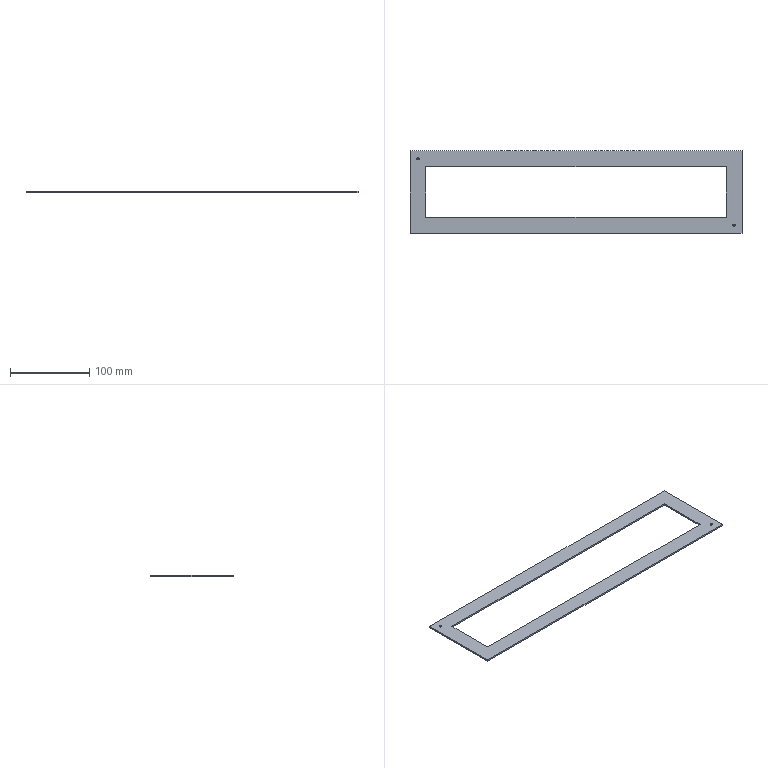Part | STEP file | Trunking Spacer Plate | 1 solid | 14 faces | box 420 x 104 x 2 mm | volume 38692 mm3 | plane 10 | cylinder 4 | commonest cylinder face diameters 3 x4
STEP:
#1=CARTESIAN_POINT('',(1421.716,-975.567,-2.));
#2=VERTEX_POINT('',#1);
#3=CARTESIAN_POINT('',(1418.716,-975.567,-2.));
#4=VERTEX_POINT('',#3);
#5=CARTESIAN_POINT('',(1420.216,-975.567,-2.));
#6=DIRECTION('',(0.,0.,-1.));
#7=DIRECTION('',(1.,0.,0.));
#8=AXIS2_PLACEMENT_3D('',#5,#6,#7);
#9=CIRCLE('',#8,1.5);
#10=EDGE_CURVE('',#2,#4,#9,.T.);
#11=ORIENTED_EDGE('',*,*,#10,.T.);
#12=CARTESIAN_POINT('',(1418.716,-975.567,0.));
#13=VERTEX_POINT('',#12);
#14=CARTESIAN_POINT('',(1418.716,-975.567,-2.));
#15=DIRECTION('',(0.,0.,1.));
#16=VECTOR('',#15,1000.);
#17=LINE('',#14,#16);
#18=EDGE_CURVE('',#4,#13,#17,.T.);
#19=ORIENTED_EDGE('',*,*,#18,.T.);
#20=CARTESIAN_POINT('',(1421.716,-975.567,0.));
#21=VERTEX_POINT('',#20);
#22=CARTESIAN_POINT('',(1420.216,-975.567,0.));
#23=DIRECTION('',(0.,0.,-1.));
#24=DIRECTION('',(1.,0.,0.));
#25=AXIS2_PLACEMENT_3D('',#22,#23,#24);
#26=CIRCLE('',#25,1.5);
#27=EDGE_CURVE('',#21,#13,#26,.T.);
#28=ORIENTED_EDGE('',*,*,#27,.F.);
#29=CARTESIAN_POINT('',(1421.716,-975.567,-2.));
#30=DIRECTION('',(0.,0.,1.));
#31=VECTOR('',#30,1000.);
#32=LINE('',#29,#31);
#33=EDGE_CURVE('',#2,#21,#32,.T.);
#34=ORIENTED_EDGE('',*,*,#33,.F.);
#35=EDGE_LOOP('',(#11,#19,#28,#34));
#36=FACE_OUTER_BOUND('',#35,.T.);
#37=CARTESIAN_POINT('',(1420.216,-975.567,-2.));
#38=DIRECTION('',(0.,0.,1.));
#39=DIRECTION('',(1.,0.,0.));
#40=AXIS2_PLACEMENT_3D('',#37,#38,#39);
#41=CYLINDRICAL_SURFACE('',#40,1.5);
#42=ADVANCED_FACE('',(#36),#41,.F.);
#43=CARTESIAN_POINT('',(1021.716,-891.567,-2.));
#44=VERTEX_POINT('',#43);
#45=CARTESIAN_POINT('',(1018.716,-891.567,-2.));
#46=VERTEX_POINT('',#45);
#47=CARTESIAN_POINT('',(1020.216,-891.567,-2.));
#48=DIRECTION('',(0.,0.,-1.));
#49=DIRECTION('',(1.,0.,0.));
#50=AXIS2_PLACEMENT_3D('',#47,#48,#49);
#51=CIRCLE('',#50,1.5);
#52=EDGE_CURVE('',#44,#46,#51,.T.);
#53=ORIENTED_EDGE('',*,*,#52,.T.);
#54=CARTESIAN_POINT('',(1018.716,-891.567,0.));
#55=VERTEX_POINT('',#54);
#56=CARTESIAN_POINT('',(1018.716,-891.567,-2.));
#57=DIRECTION('',(0.,0.,1.));
#58=VECTOR('',#57,1000.);
#59=LINE('',#56,#58);
#60=EDGE_CURVE('',#46,#55,#59,.T.);
#61=ORIENTED_EDGE('',*,*,#60,.T.);
#62=CARTESIAN_POINT('',(1021.716,-891.567,0.));
#63=VERTEX_POINT('',#62);
#64=CARTESIAN_POINT('',(1020.216,-891.567,0.));
#65=DIRECTION('',(0.,0.,-1.));
#66=DIRECTION('',(1.,0.,0.));
#67=AXIS2_PLACEMENT_3D('',#64,#65,#66);
#68=CIRCLE('',#67,1.5);
#69=EDGE_CURVE('',#63,#55,#68,.T.);
#70=ORIENTED_EDGE('',*,*,#69,.F.);
#71=CARTESIAN_POINT('',(1021.716,-891.567,-2.));
#72=DIRECTION('',(0.,0.,1.));
#73=VECTOR('',#72,1000.);
#74=LINE('',#71,#73);
#75=EDGE_CURVE('',#44,#63,#74,.T.);
#76=ORIENTED_EDGE('',*,*,#75,.F.);
#77=EDGE_LOOP('',(#53,#61,#70,#76));
#78=FACE_OUTER_BOUND('',#77,.T.);
#79=CARTESIAN_POINT('',(1020.216,-891.567,-2.));
#80=DIRECTION('',(0.,0.,1.));
#81=DIRECTION('',(1.,0.,0.));
#82=AXIS2_PLACEMENT_3D('',#79,#80,#81);
#83=CYLINDRICAL_SURFACE('',#82,1.5);
#84=ADVANCED_FACE('',(#78),#83,.F.);
#85=CARTESIAN_POINT('',(1430.216,-881.567,-2.));
#86=VERTEX_POINT('',#85);
#87=CARTESIAN_POINT('',(1010.216,-881.567,-2.));
#88=VERTEX_POINT('',#87);
#89=CARTESIAN_POINT('',(0.,-881.567,-2.));
#90=DIRECTION('',(-1.,0.,0.));
#91=VECTOR('',#90,1000.);
#92=LINE('',#89,#91);
#93=EDGE_CURVE('',#86,#88,#92,.T.);
#94=ORIENTED_EDGE('',*,*,#93,.F.);
#95=CARTESIAN_POINT('',(1430.216,-985.567,-2.));
#96=VERTEX_POINT('',#95);
#97=CARTESIAN_POINT('',(1430.216,0.,-2.));
#98=DIRECTION('',(0.,1.,0.));
#99=VECTOR('',#98,1000.);
#100=LINE('',#97,#99);
#101=EDGE_CURVE('',#96,#86,#100,.T.);
#102=ORIENTED_EDGE('',*,*,#101,.F.);
#103=CARTESIAN_POINT('',(1010.216,-985.567,-2.));
#104=VERTEX_POINT('',#103);
#105=CARTESIAN_POINT('',(0.,-985.567,-2.));
#106=DIRECTION('',(1.,0.,0.));
#107=VECTOR('',#106,1000.);
#108=LINE('',#105,#107);
#109=EDGE_CURVE('',#104,#96,#108,.T.);
#110=ORIENTED_EDGE('',*,*,#109,.F.);
#111=CARTESIAN_POINT('',(1010.216,0.,-2.));
#112=DIRECTION('',(0.,-1.,0.));
#113=VECTOR('',#112,1000.);
#114=LINE('',#111,#113);
#115=EDGE_CURVE('',#88,#104,#114,.T.);
#116=ORIENTED_EDGE('',*,*,#115,.F.);
#117=EDGE_LOOP('',(#94,#102,#110,#116));
#118=FACE_OUTER_BOUND('',#117,.T.);
#119=ORIENTED_EDGE('',*,*,#10,.F.);
#120=CARTESIAN_POINT('',(1420.216,-975.567,-2.));
#121=DIRECTION('',(0.,0.,-1.));
#122=DIRECTION('',(1.,0.,0.));
#123=AXIS2_PLACEMENT_3D('',#120,#121,#122);
#124=CIRCLE('',#123,1.5);
#125=EDGE_CURVE('',#4,#2,#124,.T.);
#126=ORIENTED_EDGE('',*,*,#125,.F.);
#127=EDGE_LOOP('',(#119,#126));
#128=FACE_BOUND('',#127,.T.);
#129=ORIENTED_EDGE('',*,*,#52,.F.);
#130=CARTESIAN_POINT('',(1020.216,-891.567,-2.));
#131=DIRECTION('',(0.,0.,-1.));
#132=DIRECTION('',(1.,0.,0.));
#133=AXIS2_PLACEMENT_3D('',#130,#131,#132);
#134=CIRCLE('',#133,1.5);
#135=EDGE_CURVE('',#46,#44,#134,.T.);
#136=ORIENTED_EDGE('',*,*,#135,.F.);
#137=EDGE_LOOP('',(#129,#136));
#138=FACE_BOUND('',#137,.T.);
#139=CARTESIAN_POINT('',(1030.216,-965.567,-2.));
#140=VERTEX_POINT('',#139);
#141=CARTESIAN_POINT('',(1030.216,-901.567,-2.));
#142=VERTEX_POINT('',#141);
#143=CARTESIAN_POINT('',(1030.216,0.,-2.));
#144=DIRECTION('',(0.,1.,0.));
#145=VECTOR('',#144,1000.);
#146=LINE('',#143,#145);
#147=EDGE_CURVE('',#140,#142,#146,.T.);
#148=ORIENTED_EDGE('',*,*,#147,.F.);
#149=CARTESIAN_POINT('',(1410.216,-965.567,-2.));
#150=VERTEX_POINT('',#149);
#151=CARTESIAN_POINT('',(0.,-965.567,-2.));
#152=DIRECTION('',(-1.,0.,0.));
#153=VECTOR('',#152,1000.);
#154=LINE('',#151,#153);
#155=EDGE_CURVE('',#150,#140,#154,.T.);
#156=ORIENTED_EDGE('',*,*,#155,.F.);
#157=CARTESIAN_POINT('',(1410.216,-901.567,-2.));
#158=VERTEX_POINT('',#157);
#159=CARTESIAN_POINT('',(1410.216,0.,-2.));
#160=DIRECTION('',(0.,-1.,0.));
#161=VECTOR('',#160,1000.);
#162=LINE('',#159,#161);
#163=EDGE_CURVE('',#158,#150,#162,.T.);
#164=ORIENTED_EDGE('',*,*,#163,.F.);
#165=CARTESIAN_POINT('',(0.,-901.567,-2.));
#166=DIRECTION('',(1.,0.,0.));
#167=VECTOR('',#166,1000.);
#168=LINE('',#165,#167);
#169=EDGE_CURVE('',#142,#158,#168,.T.);
#170=ORIENTED_EDGE('',*,*,#169,.F.);
#171=EDGE_LOOP('',(#148,#156,#164,#170));
#172=FACE_BOUND('',#171,.T.);
#173=CARTESIAN_POINT('',(0.,0.,-2.));
#174=DIRECTION('',(0.,0.,1.));
#175=DIRECTION('',(1.,0.,0.));
#176=AXIS2_PLACEMENT_3D('',#173,#174,#175);
#177=PLANE('',#176);
#178=ADVANCED_FACE('',(#118,#128,#138,#172),#177,.F.);
#179=ORIENTED_EDGE('',*,*,#115,.T.);
#180=CARTESIAN_POINT('',(1010.216,-985.567,0.));
#181=VERTEX_POINT('',#180);
#182=CARTESIAN_POINT('',(1010.216,-985.567,-2.));
#183=DIRECTION('',(0.,0.,1.));
#184=VECTOR('',#183,1000.);
#185=LINE('',#182,#184);
#186=EDGE_CURVE('',#104,#181,#185,.T.);
#187=ORIENTED_EDGE('',*,*,#186,.T.);
#188=CARTESIAN_POINT('',(1010.216,-881.567,0.));
#189=VERTEX_POINT('',#188);
#190=CARTESIAN_POINT('',(1010.216,-881.567,0.));
#191=DIRECTION('',(0.,1.,0.));
#192=VECTOR('',#191,1000.);
#193=LINE('',#190,#192);
#194=EDGE_CURVE('',#181,#189,#193,.T.);
#195=ORIENTED_EDGE('',*,*,#194,.T.);
#196=CARTESIAN_POINT('',(1010.216,-881.567,-2.));
#197=DIRECTION('',(0.,0.,-1.));
#198=VECTOR('',#197,1000.);
#199=LINE('',#196,#198);
#200=EDGE_CURVE('',#189,#88,#199,.T.);
#201=ORIENTED_EDGE('',*,*,#200,.T.);
#202=EDGE_LOOP('',(#179,#187,#195,#201));
#203=FACE_OUTER_BOUND('',#202,.T.);
#204=CARTESIAN_POINT('',(1010.216,-881.567,-2.));
#205=DIRECTION('',(-1.,0.,0.));
#206=DIRECTION('',(0.,-1.,0.));
#207=AXIS2_PLACEMENT_3D('',#204,#205,#206);
#208=PLANE('',#207);
#209=ADVANCED_FACE('',(#203),#208,.T.);
#210=ORIENTED_EDGE('',*,*,#93,.T.);
#211=ORIENTED_EDGE('',*,*,#200,.F.);
#212=CARTESIAN_POINT('',(1430.216,-881.567,0.));
#213=VERTEX_POINT('',#212);
#214=CARTESIAN_POINT('',(1010.216,-881.567,0.));
#215=DIRECTION('',(1.,0.,0.));
#216=VECTOR('',#215,1000.);
#217=LINE('',#214,#216);
#218=EDGE_CURVE('',#189,#213,#217,.T.);
#219=ORIENTED_EDGE('',*,*,#218,.T.);
#220=CARTESIAN_POINT('',(1430.216,-881.567,-2.));
#221=DIRECTION('',(0.,0.,-1.));
#222=VECTOR('',#221,1000.);
#223=LINE('',#220,#222);
#224=EDGE_CURVE('',#213,#86,#223,.T.);
#225=ORIENTED_EDGE('',*,*,#224,.T.);
#226=EDGE_LOOP('',(#210,#211,#219,#225));
#227=FACE_OUTER_BOUND('',#226,.T.);
#228=CARTESIAN_POINT('',(1010.216,-881.567,-2.));
#229=DIRECTION('',(0.,1.,0.));
#230=DIRECTION('',(0.,0.,1.));
#231=AXIS2_PLACEMENT_3D('',#228,#229,#230);
#232=PLANE('',#231);
#233=ADVANCED_FACE('',(#227),#232,.T.);
#234=ORIENTED_EDGE('',*,*,#101,.T.);
#235=ORIENTED_EDGE('',*,*,#224,.F.);
#236=CARTESIAN_POINT('',(1430.216,-985.567,0.));
#237=VERTEX_POINT('',#236);
#238=CARTESIAN_POINT('',(1430.216,-881.567,0.));
#239=DIRECTION('',(0.,-1.,0.));
#240=VECTOR('',#239,1000.);
#241=LINE('',#238,#240);
#242=EDGE_CURVE('',#213,#237,#241,.T.);
#243=ORIENTED_EDGE('',*,*,#242,.T.);
#244=CARTESIAN_POINT('',(1430.216,-985.567,-2.));
#245=DIRECTION('',(0.,0.,-1.));
#246=VECTOR('',#245,1000.);
#247=LINE('',#244,#246);
#248=EDGE_CURVE('',#237,#96,#247,.T.);
#249=ORIENTED_EDGE('',*,*,#248,.T.);
#250=EDGE_LOOP('',(#234,#235,#243,#249));
#251=FACE_OUTER_BOUND('',#250,.T.);
#252=CARTESIAN_POINT('',(1430.216,-881.567,-2.));
#253=DIRECTION('',(1.,0.,0.));
#254=DIRECTION('',(0.,1.,0.));
#255=AXIS2_PLACEMENT_3D('',#252,#253,#254);
#256=PLANE('',#255);
#257=ADVANCED_FACE('',(#251),#256,.T.);
#258=ORIENTED_EDGE('',*,*,#109,.T.);
#259=ORIENTED_EDGE('',*,*,#248,.F.);
#260=CARTESIAN_POINT('',(1010.216,-985.567,0.));
#261=DIRECTION('',(-1.,0.,0.));
#262=VECTOR('',#261,1000.);
#263=LINE('',#260,#262);
#264=EDGE_CURVE('',#237,#181,#263,.T.);
#265=ORIENTED_EDGE('',*,*,#264,.T.);
#266=ORIENTED_EDGE('',*,*,#186,.F.);
#267=EDGE_LOOP('',(#258,#259,#265,#266));
#268=FACE_OUTER_BOUND('',#267,.T.);
#269=CARTESIAN_POINT('',(1010.216,-985.567,-2.));
#270=DIRECTION('',(0.,-1.,0.));
#271=DIRECTION('',(0.,0.,-1.));
#272=AXIS2_PLACEMENT_3D('',#269,#270,#271);
#273=PLANE('',#272);
#274=ADVANCED_FACE('',(#268),#273,.T.);
#275=ORIENTED_EDGE('',*,*,#18,.F.);
#276=ORIENTED_EDGE('',*,*,#125,.T.);
#277=ORIENTED_EDGE('',*,*,#33,.T.);
#278=CARTESIAN_POINT('',(1420.216,-975.567,0.));
#279=DIRECTION('',(0.,0.,-1.));
#280=DIRECTION('',(1.,0.,0.));
#281=AXIS2_PLACEMENT_3D('',#278,#279,#280);
#282=CIRCLE('',#281,1.5);
#283=EDGE_CURVE('',#13,#21,#282,.T.);
#284=ORIENTED_EDGE('',*,*,#283,.F.);
#285=EDGE_LOOP('',(#275,#276,#277,#284));
#286=FACE_OUTER_BOUND('',#285,.T.);
#287=CARTESIAN_POINT('',(1420.216,-975.567,-2.));
#288=DIRECTION('',(0.,0.,1.));
#289=DIRECTION('',(1.,0.,0.));
#290=AXIS2_PLACEMENT_3D('',#287,#288,#289);
#291=CYLINDRICAL_SURFACE('',#290,1.5);
#292=ADVANCED_FACE('',(#286),#291,.F.);
#293=ORIENTED_EDGE('',*,*,#60,.F.);
#294=ORIENTED_EDGE('',*,*,#135,.T.);
#295=ORIENTED_EDGE('',*,*,#75,.T.);
#296=CARTESIAN_POINT('',(1020.216,-891.567,0.));
#297=DIRECTION('',(0.,0.,-1.));
#298=DIRECTION('',(1.,0.,0.));
#299=AXIS2_PLACEMENT_3D('',#296,#297,#298);
#300=CIRCLE('',#299,1.5);
#301=EDGE_CURVE('',#55,#63,#300,.T.);
#302=ORIENTED_EDGE('',*,*,#301,.F.);
#303=EDGE_LOOP('',(#293,#294,#295,#302));
#304=FACE_OUTER_BOUND('',#303,.T.);
#305=CARTESIAN_POINT('',(1020.216,-891.567,-2.));
#306=DIRECTION('',(0.,0.,1.));
#307=DIRECTION('',(1.,0.,0.));
#308=AXIS2_PLACEMENT_3D('',#305,#306,#307);
#309=CYLINDRICAL_SURFACE('',#308,1.5);
#310=ADVANCED_FACE('',(#304),#309,.F.);
#311=CARTESIAN_POINT('',(1030.216,-901.567,0.));
#312=VERTEX_POINT('',#311);
#313=CARTESIAN_POINT('',(1030.216,-901.567,-2.));
#314=DIRECTION('',(0.,0.,1.));
#315=VECTOR('',#314,1000.);
#316=LINE('',#313,#315);
#317=EDGE_CURVE('',#142,#312,#316,.T.);
#318=ORIENTED_EDGE('',*,*,#317,.F.);
#319=ORIENTED_EDGE('',*,*,#169,.T.);
#320=CARTESIAN_POINT('',(1410.216,-901.567,0.));
#321=VERTEX_POINT('',#320);
#322=CARTESIAN_POINT('',(1410.216,-901.567,-2.));
#323=DIRECTION('',(0.,0.,-1.));
#324=VECTOR('',#323,1000.);
#325=LINE('',#322,#324);
#326=EDGE_CURVE('',#321,#158,#325,.T.);
#327=ORIENTED_EDGE('',*,*,#326,.F.);
#328=CARTESIAN_POINT('',(1030.216,-901.567,0.));
#329=DIRECTION('',(1.,0.,0.));
#330=VECTOR('',#329,1000.);
#331=LINE('',#328,#330);
#332=EDGE_CURVE('',#312,#321,#331,.T.);
#333=ORIENTED_EDGE('',*,*,#332,.F.);
#334=EDGE_LOOP('',(#318,#319,#327,#333));
#335=FACE_OUTER_BOUND('',#334,.T.);
#336=CARTESIAN_POINT('',(1030.216,-901.567,-2.));
#337=DIRECTION('',(0.,1.,0.));
#338=DIRECTION('',(0.,0.,1.));
#339=AXIS2_PLACEMENT_3D('',#336,#337,#338);
#340=PLANE('',#339);
#341=ADVANCED_FACE('',(#335),#340,.F.);
#342=CARTESIAN_POINT('',(1030.216,-965.567,0.));
#343=VERTEX_POINT('',#342);
#344=CARTESIAN_POINT('',(1030.216,-965.567,-2.));
#345=DIRECTION('',(0.,0.,1.));
#346=VECTOR('',#345,1000.);
#347=LINE('',#344,#346);
#348=EDGE_CURVE('',#140,#343,#347,.T.);
#349=ORIENTED_EDGE('',*,*,#348,.F.);
#350=ORIENTED_EDGE('',*,*,#147,.T.);
#351=ORIENTED_EDGE('',*,*,#317,.T.);
#352=CARTESIAN_POINT('',(1030.216,-901.567,0.));
#353=DIRECTION('',(0.,1.,0.));
#354=VECTOR('',#353,1000.);
#355=LINE('',#352,#354);
#356=EDGE_CURVE('',#343,#312,#355,.T.);
#357=ORIENTED_EDGE('',*,*,#356,.F.);
#358=EDGE_LOOP('',(#349,#350,#351,#357));
#359=FACE_OUTER_BOUND('',#358,.T.);
#360=CARTESIAN_POINT('',(1030.216,-901.567,-2.));
#361=DIRECTION('',(-1.,0.,0.));
#362=DIRECTION('',(0.,0.,1.));
#363=AXIS2_PLACEMENT_3D('',#360,#361,#362);
#364=PLANE('',#363);
#365=ADVANCED_FACE('',(#359),#364,.F.);
#366=CARTESIAN_POINT('',(1410.216,-965.567,0.));
#367=VERTEX_POINT('',#366);
#368=CARTESIAN_POINT('',(1410.216,-965.567,-2.));
#369=DIRECTION('',(0.,0.,1.));
#370=VECTOR('',#369,1000.);
#371=LINE('',#368,#370);
#372=EDGE_CURVE('',#150,#367,#371,.T.);
#373=ORIENTED_EDGE('',*,*,#372,.F.);
#374=ORIENTED_EDGE('',*,*,#155,.T.);
#375=ORIENTED_EDGE('',*,*,#348,.T.);
#376=CARTESIAN_POINT('',(1030.216,-965.567,0.));
#377=DIRECTION('',(-1.,0.,0.));
#378=VECTOR('',#377,1000.);
#379=LINE('',#376,#378);
#380=EDGE_CURVE('',#367,#343,#379,.T.);
#381=ORIENTED_EDGE('',*,*,#380,.F.);
#382=EDGE_LOOP('',(#373,#374,#375,#381));
#383=FACE_OUTER_BOUND('',#382,.T.);
#384=CARTESIAN_POINT('',(1030.216,-965.567,-2.));
#385=DIRECTION('',(0.,-1.,0.));
#386=DIRECTION('',(0.,0.,-1.));
#387=AXIS2_PLACEMENT_3D('',#384,#385,#386);
#388=PLANE('',#387);
#389=ADVANCED_FACE('',(#383),#388,.F.);
#390=ORIENTED_EDGE('',*,*,#326,.T.);
#391=ORIENTED_EDGE('',*,*,#163,.T.);
#392=ORIENTED_EDGE('',*,*,#372,.T.);
#393=CARTESIAN_POINT('',(1410.216,-901.567,0.));
#394=DIRECTION('',(0.,-1.,0.));
#395=VECTOR('',#394,1000.);
#396=LINE('',#393,#395);
#397=EDGE_CURVE('',#321,#367,#396,.T.);
#398=ORIENTED_EDGE('',*,*,#397,.F.);
#399=EDGE_LOOP('',(#390,#391,#392,#398));
#400=FACE_OUTER_BOUND('',#399,.T.);
#401=CARTESIAN_POINT('',(1410.216,-901.567,-2.));
#402=DIRECTION('',(1.,0.,0.));
#403=DIRECTION('',(0.,0.,-1.));
#404=AXIS2_PLACEMENT_3D('',#401,#402,#403);
#405=PLANE('',#404);
#406=ADVANCED_FACE('',(#400),#405,.F.);
#407=ORIENTED_EDGE('',*,*,#242,.F.);
#408=ORIENTED_EDGE('',*,*,#218,.F.);
#409=ORIENTED_EDGE('',*,*,#194,.F.);
#410=ORIENTED_EDGE('',*,*,#264,.F.);
#411=EDGE_LOOP('',(#407,#408,#409,#410));
#412=FACE_OUTER_BOUND('',#411,.T.);
#413=ORIENTED_EDGE('',*,*,#27,.T.);
#414=ORIENTED_EDGE('',*,*,#283,.T.);
#415=EDGE_LOOP('',(#413,#414));
#416=FACE_BOUND('',#415,.T.);
#417=ORIENTED_EDGE('',*,*,#69,.T.);
#418=ORIENTED_EDGE('',*,*,#301,.T.);
#419=EDGE_LOOP('',(#417,#418));
#420=FACE_BOUND('',#419,.T.);
#421=ORIENTED_EDGE('',*,*,#397,.T.);
#422=ORIENTED_EDGE('',*,*,#380,.T.);
#423=ORIENTED_EDGE('',*,*,#356,.T.);
#424=ORIENTED_EDGE('',*,*,#332,.T.);
#425=EDGE_LOOP('',(#421,#422,#423,#424));
#426=FACE_BOUND('',#425,.T.);
#427=CARTESIAN_POINT('',(0.,0.,0.));
#428=DIRECTION('',(0.,0.,1.));
#429=DIRECTION('',(1.,0.,0.));
#430=AXIS2_PLACEMENT_3D('',#427,#428,#429);
#431=PLANE('',#430);
#432=ADVANCED_FACE('',(#412,#416,#420,#426),#431,.T.);
#433=CLOSED_SHELL('',(#42,#84,#178,#209,#233,#257,#274,#292,#310,#341,#365,#389,#406,#432));
#434=MANIFOLD_SOLID_BREP('',#433);
#435=CARTESIAN_POINT('',(0.,0.,0.));
#436=DIRECTION('',(0.,0.,1.));
#437=DIRECTION('',(1.,0.,0.));
#438=AXIS2_PLACEMENT_3D('',#435,#436,#437);
#439=(LENGTH_UNIT()NAMED_UNIT(*)SI_UNIT(.MILLI.,.METRE.));
#440=UNCERTAINTY_MEASURE_WITH_UNIT(LENGTH_MEASURE(0.00001),#439,'','');
#441=(NAMED_UNIT(*)PLANE_ANGLE_UNIT()SI_UNIT($,.RADIAN.));
#442=(NAMED_UNIT(*)SI_UNIT($,.STERADIAN.)SOLID_ANGLE_UNIT());
#443=(GEOMETRIC_REPRESENTATION_CONTEXT(3)GLOBAL_UNCERTAINTY_ASSIGNED_CONTEXT((#440))GLOBAL_UNIT_ASSIGNED_CONTEXT((#439,#441,#442))REPRESENTATION_CONTEXT('',''));
#444=ADVANCED_BREP_SHAPE_REPRESENTATION('',(#434,#438),#443);